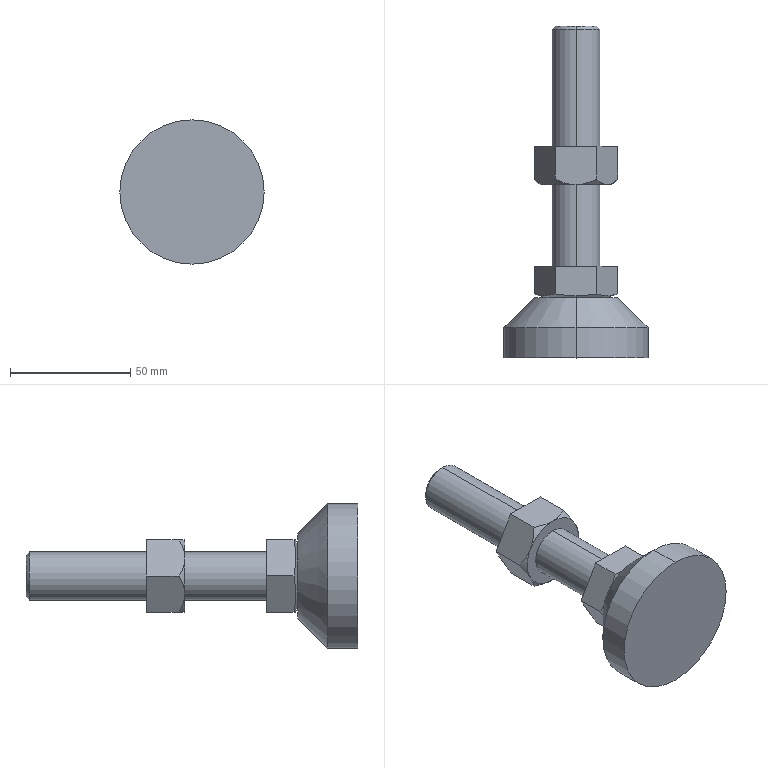Part | STEP file | Adjustable foot | 2 solids | 45 faces | box 60 x 138 x 60 mm | volume 107820 mm3 | plane 18 | cone 16 | cylinder 10 | spline 1 | commonest cylinder face diameters 17.294 x2 20 x2 27 x2 35 x2 60 x2